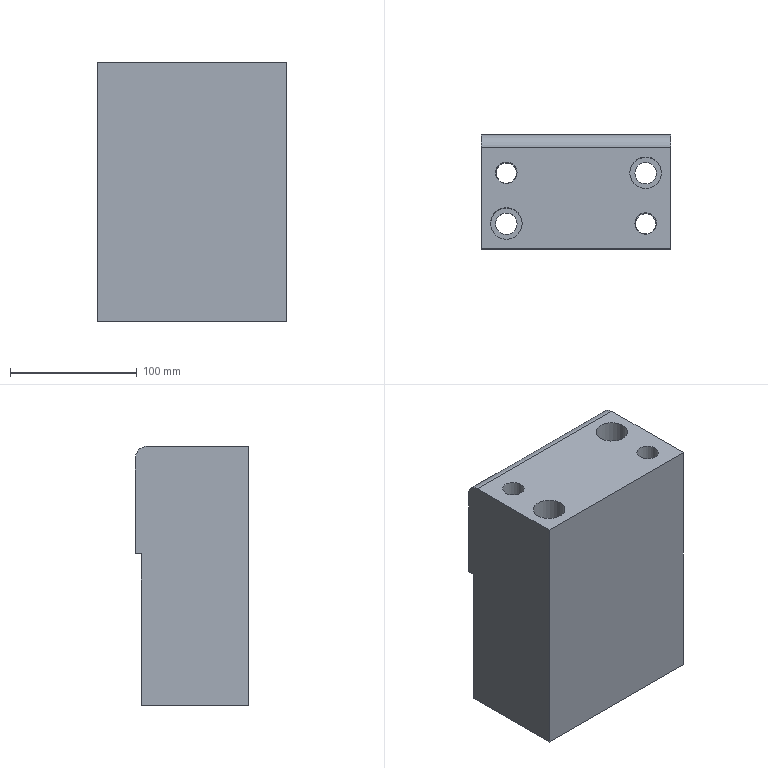Part | NX | features solid 2 | 1 solid | 21 faces | box 150 x 90 x 205 mm | volume 2397350 mm3 | plane 12 | cylinder 9 | commonest cylinder face diameters 17 x4 16 x2 25 x2 20 x1
STEP:
#1=CARTESIAN_POINT('',(-138.,-275.,-180.));
#2=VERTEX_POINT('',#1);
#3=CARTESIAN_POINT('',(-130.,-275.,-180.));
#4=DIRECTION('',(0.,0.,-1.));
#5=DIRECTION('',(-1.,0.,0.));
#6=AXIS2_PLACEMENT_3D('',#3,#4,#5);
#7=CIRCLE('',#6,8.);
#8=EDGE_CURVE('',#2,#2,#7,.T.);
#9=ORIENTED_EDGE('',*,*,#8,.F.);
#10=EDGE_LOOP('',(#9));
#11=FACE_BOUND('',#10,.T.);
#12=CARTESIAN_POINT('',(-248.,-235.,-180.));
#13=VERTEX_POINT('',#12);
#14=CARTESIAN_POINT('',(-240.,-235.,-180.));
#15=DIRECTION('',(0.,0.,-1.));
#16=DIRECTION('',(-1.,0.,0.));
#17=AXIS2_PLACEMENT_3D('',#14,#15,#16);
#18=CIRCLE('',#17,8.);
#19=EDGE_CURVE('',#13,#13,#18,.T.);
#20=ORIENTED_EDGE('',*,*,#19,.F.);
#21=EDGE_LOOP('',(#20));
#22=FACE_BOUND('',#21,.T.);
#23=CARTESIAN_POINT('',(-248.5,-275.,-180.));
#24=VERTEX_POINT('',#23);
#25=CARTESIAN_POINT('',(-240.,-275.,-180.));
#26=DIRECTION('',(0.,0.,-1.));
#27=DIRECTION('',(-1.,0.,0.));
#28=AXIS2_PLACEMENT_3D('',#25,#26,#27);
#29=CIRCLE('',#28,8.5);
#30=EDGE_CURVE('',#24,#24,#29,.T.);
#31=ORIENTED_EDGE('',*,*,#30,.F.);
#32=EDGE_LOOP('',(#31));
#33=FACE_BOUND('',#32,.T.);
#34=CARTESIAN_POINT('',(-138.5,-235.,-180.));
#35=VERTEX_POINT('',#34);
#36=CARTESIAN_POINT('',(-130.,-235.,-180.));
#37=DIRECTION('',(0.,0.,-1.));
#38=DIRECTION('',(-1.,0.,0.));
#39=AXIS2_PLACEMENT_3D('',#36,#37,#38);
#40=CIRCLE('',#39,8.5);
#41=EDGE_CURVE('',#35,#35,#40,.T.);
#42=ORIENTED_EDGE('',*,*,#41,.F.);
#43=EDGE_LOOP('',(#42));
#44=FACE_BOUND('',#43,.T.);
#45=CARTESIAN_POINT('',(-260.,-210.,-180.));
#46=VERTEX_POINT('',#45);
#47=CARTESIAN_POINT('',(-260.,-295.,-180.));
#48=VERTEX_POINT('',#47);
#49=CARTESIAN_POINT('',(-260.,-280.,-180.));
#50=DIRECTION('',(0.,-1.,0.));
#51=VECTOR('',#50,1000.);
#52=LINE('',#49,#51);
#53=EDGE_CURVE('',#46,#48,#52,.T.);
#54=ORIENTED_EDGE('',*,*,#53,.F.);
#55=CARTESIAN_POINT('',(-110.,-210.,-180.));
#56=VERTEX_POINT('',#55);
#57=CARTESIAN_POINT('',(-95.,-210.,-180.));
#58=DIRECTION('',(-1.,0.,0.));
#59=VECTOR('',#58,1000.);
#60=LINE('',#57,#59);
#61=EDGE_CURVE('',#56,#46,#60,.T.);
#62=ORIENTED_EDGE('',*,*,#61,.F.);
#63=CARTESIAN_POINT('',(-110.,-295.,-180.));
#64=VERTEX_POINT('',#63);
#65=CARTESIAN_POINT('',(-110.,-280.,-180.));
#66=DIRECTION('',(0.,-1.,0.));
#67=VECTOR('',#66,1000.);
#68=LINE('',#65,#67);
#69=EDGE_CURVE('',#56,#64,#68,.T.);
#70=ORIENTED_EDGE('',*,*,#69,.T.);
#71=CARTESIAN_POINT('',(-110.,-295.,-180.));
#72=DIRECTION('',(1.,0.,0.));
#73=VECTOR('',#72,1000.);
#74=LINE('',#71,#73);
#75=EDGE_CURVE('',#64,#48,#74,.F.);
#76=ORIENTED_EDGE('',*,*,#75,.T.);
#77=EDGE_LOOP('',(#54,#62,#70,#76));
#78=FACE_BOUND('',#77,.T.);
#79=CARTESIAN_POINT('',(-95.,-280.,-180.));
#80=DIRECTION('',(0.,0.,-1.));
#81=DIRECTION('',(-1.,0.,0.));
#82=AXIS2_PLACEMENT_3D('',#79,#80,#81);
#83=PLANE('',#82);
#84=ADVANCED_FACE('',(#11,#22,#33,#44,#78),#83,.T.);
#85=CARTESIAN_POINT('',(-260.,-210.,-60.));
#86=VERTEX_POINT('',#85);
#87=CARTESIAN_POINT('',(-260.,-210.,-170.));
#88=DIRECTION('',(0.,0.,1.));
#89=VECTOR('',#88,1000.);
#90=LINE('',#87,#89);
#91=EDGE_CURVE('',#46,#86,#90,.T.);
#92=ORIENTED_EDGE('',*,*,#91,.T.);
#93=CARTESIAN_POINT('',(-110.,-210.,-60.));
#94=VERTEX_POINT('',#93);
#95=CARTESIAN_POINT('',(-95.,-210.,-60.));
#96=DIRECTION('',(-1.,0.,0.));
#97=VECTOR('',#96,1000.);
#98=LINE('',#95,#97);
#99=EDGE_CURVE('',#94,#86,#98,.T.);
#100=ORIENTED_EDGE('',*,*,#99,.F.);
#101=CARTESIAN_POINT('',(-110.,-210.,-170.));
#102=DIRECTION('',(0.,0.,1.));
#103=VECTOR('',#102,1000.);
#104=LINE('',#101,#103);
#105=EDGE_CURVE('',#56,#94,#104,.T.);
#106=ORIENTED_EDGE('',*,*,#105,.F.);
#107=ORIENTED_EDGE('',*,*,#61,.T.);
#108=EDGE_LOOP('',(#92,#100,#106,#107));
#109=FACE_BOUND('',#108,.T.);
#110=CARTESIAN_POINT('',(-95.,-210.,-170.));
#111=DIRECTION('',(0.,-1.,0.));
#112=DIRECTION('',(0.,0.,-1.));
#113=AXIS2_PLACEMENT_3D('',#110,#111,#112);
#114=PLANE('',#113);
#115=ADVANCED_FACE('',(#109),#114,.F.);
#116=CARTESIAN_POINT('',(-260.,-295.,25.));
#117=VERTEX_POINT('',#116);
#118=CARTESIAN_POINT('',(-260.,-295.,5.));
#119=DIRECTION('',(0.,0.,1.));
#120=VECTOR('',#119,1000.);
#121=LINE('',#118,#120);
#122=EDGE_CURVE('',#117,#48,#121,.F.);
#123=ORIENTED_EDGE('',*,*,#122,.T.);
#124=ORIENTED_EDGE('',*,*,#75,.F.);
#125=CARTESIAN_POINT('',(-110.,-295.,25.));
#126=VERTEX_POINT('',#125);
#127=CARTESIAN_POINT('',(-110.,-295.,5.));
#128=DIRECTION('',(0.,0.,1.));
#129=VECTOR('',#128,1000.);
#130=LINE('',#127,#129);
#131=EDGE_CURVE('',#126,#64,#130,.F.);
#132=ORIENTED_EDGE('',*,*,#131,.F.);
#133=CARTESIAN_POINT('',(-95.,-295.,25.));
#134=DIRECTION('',(1.,0.,0.));
#135=VECTOR('',#134,1000.);
#136=LINE('',#133,#135);
#137=EDGE_CURVE('',#126,#117,#136,.F.);
#138=ORIENTED_EDGE('',*,*,#137,.T.);
#139=EDGE_LOOP('',(#123,#124,#132,#138));
#140=FACE_BOUND('',#139,.T.);
#141=CARTESIAN_POINT('',(-110.,-295.,5.));
#142=DIRECTION('',(0.,-1.,0.));
#143=DIRECTION('',(-1.,0.,0.));
#144=AXIS2_PLACEMENT_3D('',#141,#142,#143);
#145=PLANE('',#144);
#146=ADVANCED_FACE('',(#140),#145,.T.);
#147=CARTESIAN_POINT('',(-110.,-205.,-60.));
#148=VERTEX_POINT('',#147);
#149=CARTESIAN_POINT('',(-110.,-205.,15.));
#150=VERTEX_POINT('',#149);
#151=CARTESIAN_POINT('',(-110.,-205.,-70.));
#152=DIRECTION('',(0.,0.,1.));
#153=VECTOR('',#152,1000.);
#154=LINE('',#151,#153);
#155=EDGE_CURVE('',#148,#150,#154,.T.);
#156=ORIENTED_EDGE('',*,*,#155,.T.);
#157=CARTESIAN_POINT('',(-110.,-215.,25.));
#158=VERTEX_POINT('',#157);
#159=CARTESIAN_POINT('',(-110.,-215.,15.));
#160=DIRECTION('',(1.,0.,0.));
#161=DIRECTION('',(0.,0.,-1.));
#162=AXIS2_PLACEMENT_3D('',#159,#160,#161);
#163=CIRCLE('',#162,10.);
#164=EDGE_CURVE('',#150,#158,#163,.T.);
#165=ORIENTED_EDGE('',*,*,#164,.T.);
#166=CARTESIAN_POINT('',(-110.,399.,25.));
#167=DIRECTION('',(0.,1.,0.));
#168=VECTOR('',#167,1000.);
#169=LINE('',#166,#168);
#170=EDGE_CURVE('',#126,#158,#169,.T.);
#171=ORIENTED_EDGE('',*,*,#170,.F.);
#172=ORIENTED_EDGE('',*,*,#131,.T.);
#173=ORIENTED_EDGE('',*,*,#69,.F.);
#174=ORIENTED_EDGE('',*,*,#105,.T.);
#175=CARTESIAN_POINT('',(-110.,-355.,-60.));
#176=DIRECTION('',(0.,1.,0.));
#177=VECTOR('',#176,1000.);
#178=LINE('',#175,#177);
#179=EDGE_CURVE('',#94,#148,#178,.T.);
#180=ORIENTED_EDGE('',*,*,#179,.T.);
#181=EDGE_LOOP('',(#156,#165,#171,#172,#173,#174,#180));
#182=FACE_BOUND('',#181,.T.);
#183=CARTESIAN_POINT('',(-110.,-355.,-230.));
#184=DIRECTION('',(1.,0.,0.));
#185=DIRECTION('',(0.,0.,-1.));
#186=AXIS2_PLACEMENT_3D('',#183,#184,#185);
#187=PLANE('',#186);
#188=ADVANCED_FACE('',(#182),#187,.T.);
#189=CARTESIAN_POINT('',(-260.,-215.,25.));
#190=VERTEX_POINT('',#189);
#191=CARTESIAN_POINT('',(-260.,399.,25.));
#192=DIRECTION('',(0.,1.,0.));
#193=VECTOR('',#192,1000.);
#194=LINE('',#191,#193);
#195=EDGE_CURVE('',#117,#190,#194,.T.);
#196=ORIENTED_EDGE('',*,*,#195,.T.);
#197=CARTESIAN_POINT('',(-260.,-205.,15.));
#198=VERTEX_POINT('',#197);
#199=CARTESIAN_POINT('',(-260.,-215.,15.));
#200=DIRECTION('',(1.,0.,0.));
#201=DIRECTION('',(0.,0.,-1.));
#202=AXIS2_PLACEMENT_3D('',#199,#200,#201);
#203=CIRCLE('',#202,10.);
#204=EDGE_CURVE('',#190,#198,#203,.F.);
#205=ORIENTED_EDGE('',*,*,#204,.T.);
#206=CARTESIAN_POINT('',(-260.,-205.,-60.));
#207=VERTEX_POINT('',#206);
#208=CARTESIAN_POINT('',(-260.,-205.,-70.));
#209=DIRECTION('',(0.,0.,1.));
#210=VECTOR('',#209,1000.);
#211=LINE('',#208,#210);
#212=EDGE_CURVE('',#207,#198,#211,.T.);
#213=ORIENTED_EDGE('',*,*,#212,.F.);
#214=CARTESIAN_POINT('',(-260.,-355.,-60.));
#215=DIRECTION('',(0.,1.,0.));
#216=VECTOR('',#215,1000.);
#217=LINE('',#214,#216);
#218=EDGE_CURVE('',#86,#207,#217,.T.);
#219=ORIENTED_EDGE('',*,*,#218,.F.);
#220=ORIENTED_EDGE('',*,*,#91,.F.);
#221=ORIENTED_EDGE('',*,*,#53,.T.);
#222=ORIENTED_EDGE('',*,*,#122,.F.);
#223=EDGE_LOOP('',(#196,#205,#213,#219,#220,#221,#222));
#224=FACE_BOUND('',#223,.T.);
#225=CARTESIAN_POINT('',(-260.,-355.,-230.));
#226=DIRECTION('',(1.,0.,0.));
#227=DIRECTION('',(0.,0.,-1.));
#228=AXIS2_PLACEMENT_3D('',#225,#226,#227);
#229=PLANE('',#228);
#230=ADVANCED_FACE('',(#224),#229,.F.);
#231=CARTESIAN_POINT('',(-121.5,-275.,25.));
#232=VERTEX_POINT('',#231);
#233=CARTESIAN_POINT('',(-130.,-275.,25.));
#234=DIRECTION('',(0.,0.,1.));
#235=DIRECTION('',(1.,0.,0.));
#236=AXIS2_PLACEMENT_3D('',#233,#234,#235);
#237=CIRCLE('',#236,8.5);
#238=EDGE_CURVE('',#232,#232,#237,.T.);
#239=ORIENTED_EDGE('',*,*,#238,.F.);
#240=EDGE_LOOP('',(#239));
#241=FACE_BOUND('',#240,.T.);
#242=CARTESIAN_POINT('',(-231.5,-235.,25.));
#243=VERTEX_POINT('',#242);
#244=CARTESIAN_POINT('',(-240.,-235.,25.));
#245=DIRECTION('',(0.,0.,1.));
#246=DIRECTION('',(1.,0.,0.));
#247=AXIS2_PLACEMENT_3D('',#244,#245,#246);
#248=CIRCLE('',#247,8.5);
#249=EDGE_CURVE('',#243,#243,#248,.T.);
#250=ORIENTED_EDGE('',*,*,#249,.F.);
#251=EDGE_LOOP('',(#250));
#252=FACE_BOUND('',#251,.T.);
#253=CARTESIAN_POINT('',(-227.5,-275.,25.));
#254=VERTEX_POINT('',#253);
#255=CARTESIAN_POINT('',(-240.,-275.,25.));
#256=DIRECTION('',(0.,0.,1.));
#257=DIRECTION('',(1.,0.,0.));
#258=AXIS2_PLACEMENT_3D('',#255,#256,#257);
#259=CIRCLE('',#258,12.5);
#260=EDGE_CURVE('',#254,#254,#259,.T.);
#261=ORIENTED_EDGE('',*,*,#260,.F.);
#262=EDGE_LOOP('',(#261));
#263=FACE_BOUND('',#262,.T.);
#264=CARTESIAN_POINT('',(-117.5,-235.,25.));
#265=VERTEX_POINT('',#264);
#266=CARTESIAN_POINT('',(-130.,-235.,25.));
#267=DIRECTION('',(0.,0.,1.));
#268=DIRECTION('',(1.,0.,0.));
#269=AXIS2_PLACEMENT_3D('',#266,#267,#268);
#270=CIRCLE('',#269,12.5);
#271=EDGE_CURVE('',#265,#265,#270,.T.);
#272=ORIENTED_EDGE('',*,*,#271,.F.);
#273=EDGE_LOOP('',(#272));
#274=FACE_BOUND('',#273,.T.);
#275=ORIENTED_EDGE('',*,*,#170,.T.);
#276=CARTESIAN_POINT('',(-95.,-215.,25.));
#277=DIRECTION('',(-1.,0.,0.));
#278=VECTOR('',#277,1000.);
#279=LINE('',#276,#278);
#280=EDGE_CURVE('',#158,#190,#279,.T.);
#281=ORIENTED_EDGE('',*,*,#280,.T.);
#282=ORIENTED_EDGE('',*,*,#195,.F.);
#283=ORIENTED_EDGE('',*,*,#137,.F.);
#284=EDGE_LOOP('',(#275,#281,#282,#283));
#285=FACE_BOUND('',#284,.T.);
#286=CARTESIAN_POINT('',(-95.,399.,25.));
#287=DIRECTION('',(0.,0.,1.));
#288=DIRECTION('',(1.,0.,0.));
#289=AXIS2_PLACEMENT_3D('',#286,#287,#288);
#290=PLANE('',#289);
#291=ADVANCED_FACE('',(#241,#252,#263,#274,#285),#290,.T.);
#292=ORIENTED_EDGE('',*,*,#99,.T.);
#293=ORIENTED_EDGE('',*,*,#218,.T.);
#294=CARTESIAN_POINT('',(-95.,-205.,-60.));
#295=DIRECTION('',(-1.,0.,0.));
#296=VECTOR('',#295,1000.);
#297=LINE('',#294,#296);
#298=EDGE_CURVE('',#148,#207,#297,.T.);
#299=ORIENTED_EDGE('',*,*,#298,.F.);
#300=ORIENTED_EDGE('',*,*,#179,.F.);
#301=EDGE_LOOP('',(#292,#293,#299,#300));
#302=FACE_BOUND('',#301,.T.);
#303=CARTESIAN_POINT('',(-95.,-225.,-60.));
#304=DIRECTION('',(0.,0.,-1.));
#305=DIRECTION('',(-1.,0.,0.));
#306=AXIS2_PLACEMENT_3D('',#303,#304,#305);
#307=PLANE('',#306);
#308=ADVANCED_FACE('',(#302),#307,.T.);
#309=ORIENTED_EDGE('',*,*,#212,.T.);
#310=CARTESIAN_POINT('',(-95.,-205.,15.));
#311=DIRECTION('',(-1.,0.,0.));
#312=VECTOR('',#311,1000.);
#313=LINE('',#310,#312);
#314=EDGE_CURVE('',#198,#150,#313,.F.);
#315=ORIENTED_EDGE('',*,*,#314,.T.);
#316=ORIENTED_EDGE('',*,*,#155,.F.);
#317=ORIENTED_EDGE('',*,*,#298,.T.);
#318=EDGE_LOOP('',(#309,#315,#316,#317));
#319=FACE_BOUND('',#318,.T.);
#320=CARTESIAN_POINT('',(-95.,-205.,-70.));
#321=DIRECTION('',(0.,1.,0.));
#322=DIRECTION('',(0.,0.,1.));
#323=AXIS2_PLACEMENT_3D('',#320,#321,#322);
#324=PLANE('',#323);
#325=ADVANCED_FACE('',(#319),#324,.T.);
#326=ORIENTED_EDGE('',*,*,#164,.F.);
#327=ORIENTED_EDGE('',*,*,#314,.F.);
#328=ORIENTED_EDGE('',*,*,#204,.F.);
#329=ORIENTED_EDGE('',*,*,#280,.F.);
#330=EDGE_LOOP('',(#326,#327,#328,#329));
#331=FACE_BOUND('',#330,.T.);
#332=CARTESIAN_POINT('',(-95.,-215.,15.));
#333=DIRECTION('',(-1.,0.,0.));
#334=DIRECTION('',(0.,0.,1.));
#335=AXIS2_PLACEMENT_3D('',#332,#333,#334);
#336=CYLINDRICAL_SURFACE('',#335,10.);
#337=ADVANCED_FACE('',(#331),#336,.T.);
#338=ORIENTED_EDGE('',*,*,#41,.T.);
#339=EDGE_LOOP('',(#338));
#340=FACE_BOUND('',#339,.T.);
#341=CARTESIAN_POINT('',(-138.5,-235.,-150.));
#342=VERTEX_POINT('',#341);
#343=CARTESIAN_POINT('',(-130.,-235.,-150.));
#344=DIRECTION('',(0.,0.,-1.));
#345=DIRECTION('',(-1.,0.,0.));
#346=AXIS2_PLACEMENT_3D('',#343,#344,#345);
#347=CIRCLE('',#346,8.5);
#348=EDGE_CURVE('',#342,#342,#347,.F.);
#349=ORIENTED_EDGE('',*,*,#348,.T.);
#350=EDGE_LOOP('',(#349));
#351=FACE_BOUND('',#350,.T.);
#352=CARTESIAN_POINT('',(-130.,-235.,-210.));
#353=DIRECTION('',(0.,0.,1.));
#354=DIRECTION('',(1.,0.,0.));
#355=AXIS2_PLACEMENT_3D('',#352,#353,#354);
#356=CYLINDRICAL_SURFACE('',#355,8.5);
#357=ADVANCED_FACE('',(#340,#351),#356,.F.);
#358=ORIENTED_EDGE('',*,*,#348,.F.);
#359=EDGE_LOOP('',(#358));
#360=FACE_BOUND('',#359,.T.);
#361=CARTESIAN_POINT('',(-117.5,-235.,-150.));
#362=VERTEX_POINT('',#361);
#363=CARTESIAN_POINT('',(-130.,-235.,-150.));
#364=DIRECTION('',(0.,0.,1.));
#365=DIRECTION('',(1.,0.,0.));
#366=AXIS2_PLACEMENT_3D('',#363,#364,#365);
#367=CIRCLE('',#366,12.5);
#368=EDGE_CURVE('',#362,#362,#367,.T.);
#369=ORIENTED_EDGE('',*,*,#368,.T.);
#370=EDGE_LOOP('',(#369));
#371=FACE_BOUND('',#370,.T.);
#372=CARTESIAN_POINT('',(-130.,-235.,-150.));
#373=DIRECTION('',(0.,0.,-1.));
#374=DIRECTION('',(-1.,0.,0.));
#375=AXIS2_PLACEMENT_3D('',#372,#373,#374);
#376=PLANE('',#375);
#377=ADVANCED_FACE('',(#360,#371),#376,.F.);
#378=ORIENTED_EDGE('',*,*,#271,.T.);
#379=EDGE_LOOP('',(#378));
#380=FACE_BOUND('',#379,.T.);
#381=ORIENTED_EDGE('',*,*,#368,.F.);
#382=EDGE_LOOP('',(#381));
#383=FACE_BOUND('',#382,.T.);
#384=CARTESIAN_POINT('',(-130.,-235.,-150.));
#385=DIRECTION('',(0.,0.,1.));
#386=DIRECTION('',(1.,0.,0.));
#387=AXIS2_PLACEMENT_3D('',#384,#385,#386);
#388=CYLINDRICAL_SURFACE('',#387,12.5);
#389=ADVANCED_FACE('',(#380,#383),#388,.F.);
#390=ORIENTED_EDGE('',*,*,#30,.T.);
#391=EDGE_LOOP('',(#390));
#392=FACE_BOUND('',#391,.T.);
#393=CARTESIAN_POINT('',(-248.5,-275.,-150.));
#394=VERTEX_POINT('',#393);
#395=CARTESIAN_POINT('',(-240.,-275.,-150.));
#396=DIRECTION('',(0.,0.,-1.));
#397=DIRECTION('',(-1.,0.,0.));
#398=AXIS2_PLACEMENT_3D('',#395,#396,#397);
#399=CIRCLE('',#398,8.5);
#400=EDGE_CURVE('',#394,#394,#399,.F.);
#401=ORIENTED_EDGE('',*,*,#400,.T.);
#402=EDGE_LOOP('',(#401));
#403=FACE_BOUND('',#402,.T.);
#404=CARTESIAN_POINT('',(-240.,-275.,-210.));
#405=DIRECTION('',(0.,0.,1.));
#406=DIRECTION('',(1.,0.,0.));
#407=AXIS2_PLACEMENT_3D('',#404,#405,#406);
#408=CYLINDRICAL_SURFACE('',#407,8.5);
#409=ADVANCED_FACE('',(#392,#403),#408,.F.);
#410=ORIENTED_EDGE('',*,*,#400,.F.);
#411=EDGE_LOOP('',(#410));
#412=FACE_BOUND('',#411,.T.);
#413=CARTESIAN_POINT('',(-227.5,-275.,-150.));
#414=VERTEX_POINT('',#413);
#415=CARTESIAN_POINT('',(-240.,-275.,-150.));
#416=DIRECTION('',(0.,0.,1.));
#417=DIRECTION('',(1.,0.,0.));
#418=AXIS2_PLACEMENT_3D('',#415,#416,#417);
#419=CIRCLE('',#418,12.5);
#420=EDGE_CURVE('',#414,#414,#419,.T.);
#421=ORIENTED_EDGE('',*,*,#420,.T.);
#422=EDGE_LOOP('',(#421));
#423=FACE_BOUND('',#422,.T.);
#424=CARTESIAN_POINT('',(-240.,-275.,-150.));
#425=DIRECTION('',(0.,0.,-1.));
#426=DIRECTION('',(-1.,0.,0.));
#427=AXIS2_PLACEMENT_3D('',#424,#425,#426);
#428=PLANE('',#427);
#429=ADVANCED_FACE('',(#412,#423),#428,.F.);
#430=ORIENTED_EDGE('',*,*,#260,.T.);
#431=EDGE_LOOP('',(#430));
#432=FACE_BOUND('',#431,.T.);
#433=ORIENTED_EDGE('',*,*,#420,.F.);
#434=EDGE_LOOP('',(#433));
#435=FACE_BOUND('',#434,.T.);
#436=CARTESIAN_POINT('',(-240.,-275.,-150.));
#437=DIRECTION('',(0.,0.,1.));
#438=DIRECTION('',(1.,0.,0.));
#439=AXIS2_PLACEMENT_3D('',#436,#437,#438);
#440=CYLINDRICAL_SURFACE('',#439,12.5);
#441=ADVANCED_FACE('',(#432,#435),#440,.F.);
#442=ORIENTED_EDGE('',*,*,#19,.T.);
#443=EDGE_LOOP('',(#442));
#444=FACE_BOUND('',#443,.T.);
#445=CARTESIAN_POINT('',(-248.,-235.,-150.));
#446=VERTEX_POINT('',#445);
#447=CARTESIAN_POINT('',(-240.,-235.,-150.));
#448=DIRECTION('',(0.,0.,-1.));
#449=DIRECTION('',(-1.,0.,0.));
#450=AXIS2_PLACEMENT_3D('',#447,#448,#449);
#451=CIRCLE('',#450,8.);
#452=EDGE_CURVE('',#446,#446,#451,.F.);
#453=ORIENTED_EDGE('',*,*,#452,.T.);
#454=EDGE_LOOP('',(#453));
#455=FACE_BOUND('',#454,.T.);
#456=CARTESIAN_POINT('',(-240.,-235.,-210.));
#457=DIRECTION('',(0.,0.,1.));
#458=DIRECTION('',(1.,0.,0.));
#459=AXIS2_PLACEMENT_3D('',#456,#457,#458);
#460=CYLINDRICAL_SURFACE('',#459,8.);
#461=ADVANCED_FACE('',(#444,#455),#460,.F.);
#462=ORIENTED_EDGE('',*,*,#452,.F.);
#463=EDGE_LOOP('',(#462));
#464=FACE_BOUND('',#463,.T.);
#465=CARTESIAN_POINT('',(-231.5,-235.,-150.));
#466=VERTEX_POINT('',#465);
#467=CARTESIAN_POINT('',(-240.,-235.,-150.));
#468=DIRECTION('',(0.,0.,1.));
#469=DIRECTION('',(1.,0.,0.));
#470=AXIS2_PLACEMENT_3D('',#467,#468,#469);
#471=CIRCLE('',#470,8.5);
#472=EDGE_CURVE('',#466,#466,#471,.T.);
#473=ORIENTED_EDGE('',*,*,#472,.T.);
#474=EDGE_LOOP('',(#473));
#475=FACE_BOUND('',#474,.T.);
#476=CARTESIAN_POINT('',(-240.,-235.,-150.));
#477=DIRECTION('',(0.,0.,-1.));
#478=DIRECTION('',(-1.,0.,0.));
#479=AXIS2_PLACEMENT_3D('',#476,#477,#478);
#480=PLANE('',#479);
#481=ADVANCED_FACE('',(#464,#475),#480,.F.);
#482=ORIENTED_EDGE('',*,*,#249,.T.);
#483=EDGE_LOOP('',(#482));
#484=FACE_BOUND('',#483,.T.);
#485=ORIENTED_EDGE('',*,*,#472,.F.);
#486=EDGE_LOOP('',(#485));
#487=FACE_BOUND('',#486,.T.);
#488=CARTESIAN_POINT('',(-240.,-235.,-150.));
#489=DIRECTION('',(0.,0.,1.));
#490=DIRECTION('',(1.,0.,0.));
#491=AXIS2_PLACEMENT_3D('',#488,#489,#490);
#492=CYLINDRICAL_SURFACE('',#491,8.5);
#493=ADVANCED_FACE('',(#484,#487),#492,.F.);
#494=ORIENTED_EDGE('',*,*,#8,.T.);
#495=EDGE_LOOP('',(#494));
#496=FACE_BOUND('',#495,.T.);
#497=CARTESIAN_POINT('',(-138.,-275.,-150.));
#498=VERTEX_POINT('',#497);
#499=CARTESIAN_POINT('',(-130.,-275.,-150.));
#500=DIRECTION('',(0.,0.,-1.));
#501=DIRECTION('',(-1.,0.,0.));
#502=AXIS2_PLACEMENT_3D('',#499,#500,#501);
#503=CIRCLE('',#502,8.);
#504=EDGE_CURVE('',#498,#498,#503,.F.);
#505=ORIENTED_EDGE('',*,*,#504,.T.);
#506=EDGE_LOOP('',(#505));
#507=FACE_BOUND('',#506,.T.);
#508=CARTESIAN_POINT('',(-130.,-275.,-210.));
#509=DIRECTION('',(0.,0.,1.));
#510=DIRECTION('',(1.,0.,0.));
#511=AXIS2_PLACEMENT_3D('',#508,#509,#510);
#512=CYLINDRICAL_SURFACE('',#511,8.);
#513=ADVANCED_FACE('',(#496,#507),#512,.F.);
#514=ORIENTED_EDGE('',*,*,#504,.F.);
#515=EDGE_LOOP('',(#514));
#516=FACE_BOUND('',#515,.T.);
#517=CARTESIAN_POINT('',(-121.5,-275.,-150.));
#518=VERTEX_POINT('',#517);
#519=CARTESIAN_POINT('',(-130.,-275.,-150.));
#520=DIRECTION('',(0.,0.,1.));
#521=DIRECTION('',(1.,0.,0.));
#522=AXIS2_PLACEMENT_3D('',#519,#520,#521);
#523=CIRCLE('',#522,8.5);
#524=EDGE_CURVE('',#518,#518,#523,.T.);
#525=ORIENTED_EDGE('',*,*,#524,.T.);
#526=EDGE_LOOP('',(#525));
#527=FACE_BOUND('',#526,.T.);
#528=CARTESIAN_POINT('',(-130.,-275.,-150.));
#529=DIRECTION('',(0.,0.,-1.));
#530=DIRECTION('',(-1.,0.,0.));
#531=AXIS2_PLACEMENT_3D('',#528,#529,#530);
#532=PLANE('',#531);
#533=ADVANCED_FACE('',(#516,#527),#532,.F.);
#534=ORIENTED_EDGE('',*,*,#238,.T.);
#535=EDGE_LOOP('',(#534));
#536=FACE_BOUND('',#535,.T.);
#537=ORIENTED_EDGE('',*,*,#524,.F.);
#538=EDGE_LOOP('',(#537));
#539=FACE_BOUND('',#538,.T.);
#540=CARTESIAN_POINT('',(-130.,-275.,-150.));
#541=DIRECTION('',(0.,0.,1.));
#542=DIRECTION('',(1.,0.,0.));
#543=AXIS2_PLACEMENT_3D('',#540,#541,#542);
#544=CYLINDRICAL_SURFACE('',#543,8.5);
#545=ADVANCED_FACE('',(#536,#539),#544,.F.);
#546=CLOSED_SHELL('',(#84,#115,#146,#188,#230,#291,#308,#325,#337,#357,#377,#389,#409,#429,#441,#461,#481,#493,#513,#533,#545));
#547=MANIFOLD_SOLID_BREP('',#546);
#548=(LENGTH_UNIT()NAMED_UNIT(*)SI_UNIT(.MILLI.,.METRE.));
#549=UNCERTAINTY_MEASURE_WITH_UNIT(LENGTH_MEASURE(0.00001),#548,'','');
#550=(NAMED_UNIT(*)PLANE_ANGLE_UNIT()SI_UNIT($,.RADIAN.));
#551=(NAMED_UNIT(*)SI_UNIT($,.STERADIAN.)SOLID_ANGLE_UNIT());
#552=(GEOMETRIC_REPRESENTATION_CONTEXT(3)GLOBAL_UNCERTAINTY_ASSIGNED_CONTEXT((#549))GLOBAL_UNIT_ASSIGNED_CONTEXT((#548,#550,#551))REPRESENTATION_CONTEXT('',''));
#553=ADVANCED_BREP_SHAPE_REPRESENTATION('',(#547),#552);